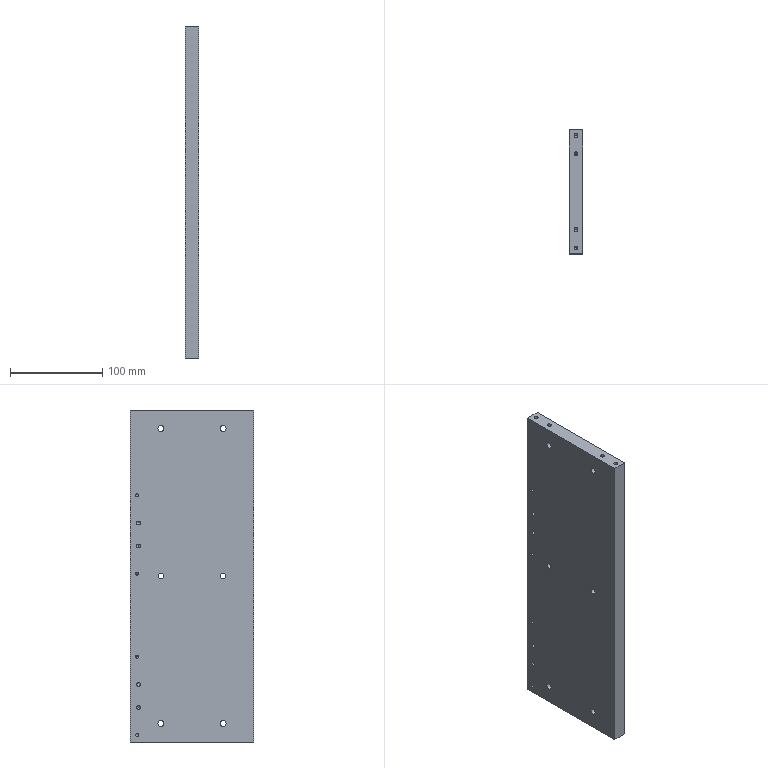Part | SolidWorks | features HoleWzd 7, LPattern 2, Extrusion 1, MirrorPattern 1 | 1 solid | 200 faces | box 15 x 134 x 360 mm | volume 714258 mm3 | cylinder 106 | cone 84 | plane 10 | commonest cylinder face diameters 3.3 x61 4.2 x25 6.6 x8 11 x8 6 x4